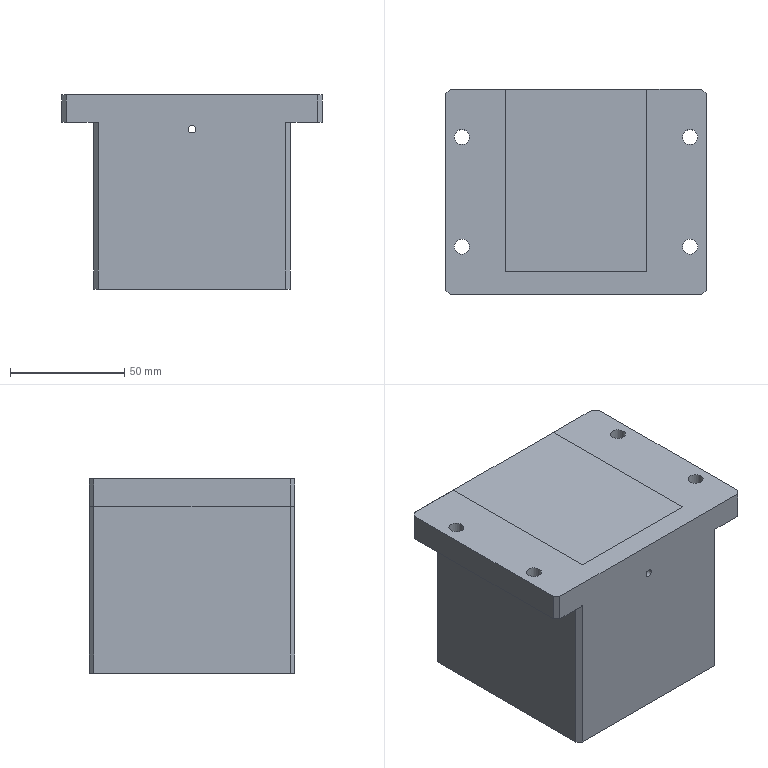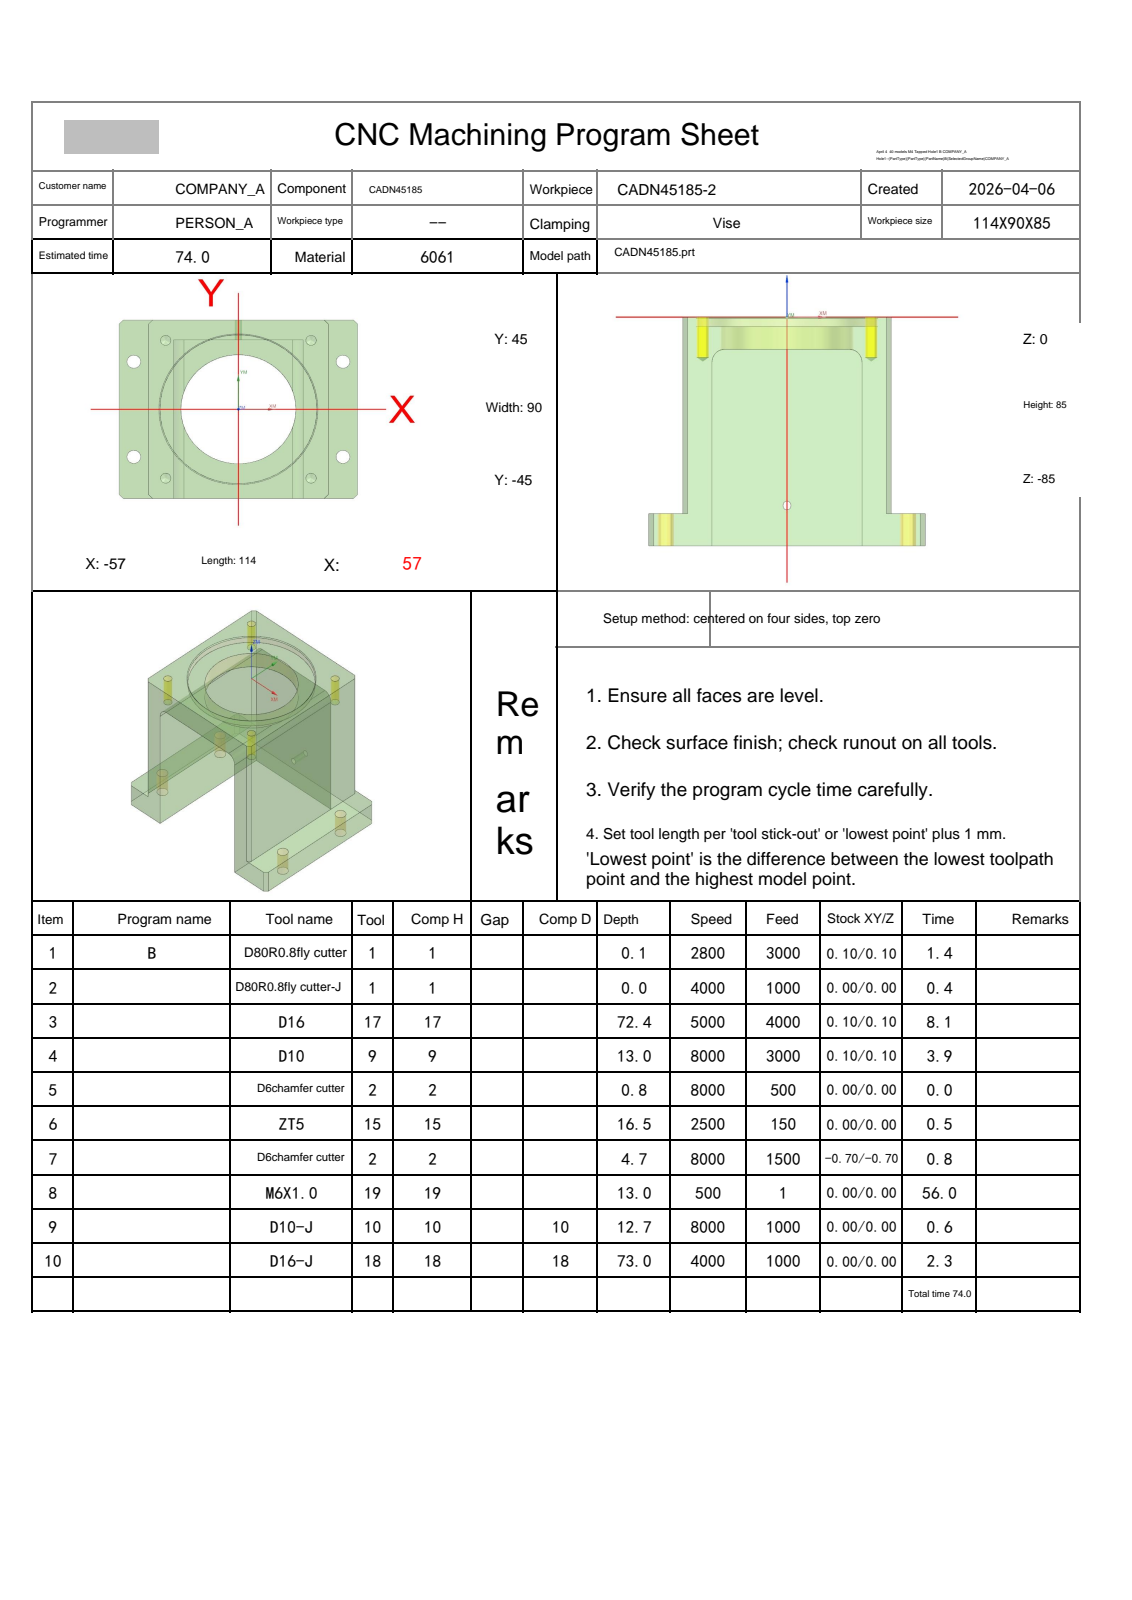NC program | NX | posted by the shop | part box 114 x 90 x 85 mm
Lines 2097 to 3620 of 3620:
N4 T09 M06
(D10  D=10. R=0. H=09 ce=0.10 di=0.10)
G00 G90 G54 X30.162 Y3.101 M03 S8000
G43 H09 Z14.5
M08
Z1.5
G02 X30.162 Y3.101 Z1.006 I-3.261 J-3.101 F3000.
X30.162 Y3.101 Z.513 I-3.261 J-3.101
X30.162 Y3.101 Z.019 I-3.261 J-3.101
X30.162 Y3.101 Z-.474 I-3.261 J-3.101
X30.583 Y2.587 Z-.486 I-3.261 J-3.101
G01 X32.401 Y0.0
G02 X0.0 Y-32.401 I-32.401 J0.0
X-32.401 Y0.0 I0.0 J32.401
X0.0 Y32.401 I32.401 J0.0
X32.401 Y0.0 I0.0 J-32.401
X32.12 Y-4.259 I-32.401 J0.0
X31.311 Y-5.111 I-.991 J.132
G01 X25.212 Y-6.237
G03 X24.433 Y-6.947 I.182 J-.983
G02 X0.0 Y-25.401 I-24.433 J6.947
X-25.401 Y0.0 I0.0 J25.401
X0.0 Y25.401 I25.401 J0.0
X25.401 Y0.0 I0.0 J-25.401
X25.388 Y-.819 I-25.401 J0.0
X24.834 Y-1.681 I-.999 J.033
G01 X18.014 Y-5.075
G03 X17.508 Y-5.662 I.446 J-.895
G02 X0.0 Y-18.401 I-17.508 J5.662
X-18.401 Y0.0 I0.0 J18.401
X0.0 Y18.401 I18.401 J0.0
X18.399 Y.3 I0.0 J-18.401
G01 Y.284
G02 X17.84 Y-.614 I-1. J0.0
G01 X10.955 Y-3.994
G03 X10.477 Y-4.497 I.441 J-.898
G02 X0.0 Y-11.401 I-10.477 J4.497
X-11.401 Y0.0 I0.0 J11.401
X0.0 Y11.401 I11.401 J0.0
X11.304 Y1.486 I0.0 J-11.401
G01 X11.312 Y1.356
G02 X10.724 Y.445 I-1. J0.0
G01 X3.487 Y-2.826
G03 X3.178 Y-3.045 I.412 J-.911
G02 X0.0 Y-4.401 I-3.178 J3.045
X-4.401 Y0.0 I0.0 J4.401
X0.0 Y4.401 I4.401 J0.0
X4.401 Y0.0 I0.0 J-4.401
X4.349 Y-.676 I-4.401 J0.0
X4.244 Y-1.165 I-4.349 J.676
G03 X3.994 Y-3.018 I6.75 J-1.853
X9.141 Y-9.768 I7. J0.0
G01 Z.714
G00 Z3.
G01 X30.161 Y3.101 F6000.
G00 Z1.014
G02 X30.161 Y3.101 Z.521 I-3.261 J-3.101 F3000.
X30.161 Y3.101 Z.027 I-3.261 J-3.101
X30.161 Y3.101 Z-.466 I-3.261 J-3.101
X30.161 Y3.101 Z-.96 I-3.261 J-3.101
X30.582 Y2.587 Z-.971 I-3.261 J-3.101
G01 X32.4 Y0.0
G02 X0.0 Y-32.4 I-32.4 J0.0
X-32.4 Y0.0 I0.0 J32.4
X0.0 Y32.4 I32.4 J0.0
X32.4 Y0.0 I0.0 J-32.4
X32.015 Y-4.98 I-32.4 J0.0
X31.108 Y-5.823 I-.988 J.154
G01 X25.292 Y-6.295
G03 X24.412 Y-7.015 I.081 J-.997
G02 X0.0 Y-25.4 I-24.412 J7.015
X-25.4 Y0.0 I0.0 J25.4
X0.0 Y25.4 I25.4 J0.0
X25.4 Y0.0 I0.0 J-25.4
X25.387 Y-.819 I-25.4 J0.0
X24.833 Y-1.681 I-.999 J.033
G01 X18.013 Y-5.075
G03 X17.507 Y-5.662 I.446 J-.895
G02 X0.0 Y-18.4 I-17.507 J5.662
X-18.4 Y0.0 I0.0 J18.4
X0.0 Y18.4 I18.4 J0.0
X18.398 Y.3 I0.0 J-18.4
G01 Y.284
G02 X17.839 Y-.614 I-1. J0.0
G01 X10.953 Y-3.994
G03 X10.476 Y-4.497 I.441 J-.897
G02 X0.0 Y-11.4 I-10.476 J4.497
X-11.4 Y0.0 I0.0 J11.4
X0.0 Y11.4 I11.4 J0.0
X11.303 Y1.486 I0.0 J-11.4
G01 X11.311 Y1.356
G02 X10.723 Y.445 I-1. J0.0
G01 X3.486 Y-2.826
G03 X3.176 Y-3.045 I.412 J-.911
G02 X0.0 Y-4.4 I-3.176 J3.045
X-4.4 Y0.0 I0.0 J4.4
X0.0 Y4.4 I4.4 J0.0
X4.4 Y0.0 I0.0 J-4.4
X4.348 Y-.676 I-4.4 J0.0
X4.243 Y-1.165 I-4.348 J.676
G03 X3.993 Y-3.018 I6.75 J-1.853
X9.14 Y-9.768 I7. J0.0
G01 Z.229
G00 Z2.514
G01 X30.161 Y3.101 F6000.
G00 Z.529
G02 X30.161 Y3.101 Z.035 I-3.261 J-3.101 F3000.
X30.161 Y3.101 Z-.458 I-3.261 J-3.101
X30.161 Y3.101 Z-.952 I-3.261 J-3.101
X30.161 Y3.101 Z-1.446 I-3.261 J-3.101
X30.582 Y2.587 Z-1.457 I-3.261 J-3.101
G01 X32.4 Y0.0
G02 X0.0 Y-32.4 I-32.4 J0.0
X-32.4 Y0.0 I0.0 J32.4
X0.0 Y32.4 I32.4 J0.0
X32.4 Y0.0 I0.0 J-32.4
X32.015 Y-4.98 I-32.4 J0.0
X31.108 Y-5.823 I-.988 J.154
G01 X25.292 Y-6.295
G03 X24.412 Y-7.015 I.081 J-.997
G02 X0.0 Y-25.4 I-24.412 J7.015
X-25.4 Y0.0 I0.0 J25.4
X0.0 Y25.4 I25.4 J0.0
X25.4 Y0.0 I0.0 J-25.4
X25.387 Y-.819 I-25.4 J0.0
X24.833 Y-1.681 I-.999 J.033
G01 X18.013 Y-5.075
G03 X17.507 Y-5.662 I.446 J-.895
G02 X0.0 Y-18.4 I-17.507 J5.662
X-18.4 Y0.0 I0.0 J18.4
X0.0 Y18.4 I18.4 J0.0
X18.398 Y.3 I0.0 J-18.4
G01 Y.284
G02 X17.839 Y-.614 I-1. J0.0
G01 X10.953 Y-3.994
G03 X10.476 Y-4.497 I.441 J-.897
G02 X0.0 Y-11.4 I-10.476 J4.497
X-11.4 Y0.0 I0.0 J11.4
X0.0 Y11.4 I11.4 J0.0
X11.303 Y1.486 I0.0 J-11.4
G01 X11.311 Y1.356
G02 X10.723 Y.445 I-1. J0.0
G01 X3.486 Y-2.826
G03 X3.176 Y-3.045 I.412 J-.911
G02 X0.0 Y-4.4 I-3.176 J3.045
X-4.4 Y0.0 I0.0 J4.4
X0.0 Y4.4 I4.4 J0.0
X4.4 Y0.0 I0.0 J-4.4
X4.348 Y-.676 I-4.4 J0.0
X4.243 Y-1.165 I-4.348 J.676
G03 X3.993 Y-3.018 I6.75 J-1.853
X9.14 Y-9.768 I7. J0.0
G01 Z-.257
G00 Z2.029
G01 X30.161 Y3.101 F6000.
G00 Z.043
G02 X30.161 Y3.101 Z-.451 I-3.261 J-3.101 F3000.
X30.161 Y3.101 Z-.944 I-3.261 J-3.101
X30.161 Y3.101 Z-1.438 I-3.261 J-3.101
X30.161 Y3.101 Z-1.931 I-3.261 J-3.101
X30.582 Y2.587 Z-1.943 I-3.261 J-3.101
G01 X32.4 Y0.0
G02 X0.0 Y-32.4 I-32.4 J0.0
X-32.4 Y0.0 I0.0 J32.4
X0.0 Y32.4 I32.4 J0.0
X32.4 Y0.0 I0.0 J-32.4
X32.015 Y-4.98 I-32.4 J0.0
X31.108 Y-5.823 I-.988 J.154
G01 X25.292 Y-6.295
G03 X24.412 Y-7.015 I.081 J-.997
G02 X0.0 Y-25.4 I-24.412 J7.015
X-25.4 Y0.0 I0.0 J25.4
X0.0 Y25.4 I25.4 J0.0
X25.4 Y0.0 I0.0 J-25.4
X25.387 Y-.819 I-25.4 J0.0
X24.833 Y-1.681 I-.999 J.033
G01 X18.013 Y-5.075
G03 X17.507 Y-5.662 I.446 J-.895
G02 X0.0 Y-18.4 I-17.507 J5.662
X-18.4 Y0.0 I0.0 J18.4
X0.0 Y18.4 I18.4 J0.0
X18.398 Y.3 I0.0 J-18.4
G01 Y.284
G02 X17.839 Y-.614 I-1. J0.0
G01 X10.953 Y-3.994
G03 X10.476 Y-4.497 I.441 J-.897
G02 X0.0 Y-11.4 I-10.476 J4.497
X-11.4 Y0.0 I0.0 J11.4
X0.0 Y11.4 I11.4 J0.0
X11.303 Y1.486 I0.0 J-11.4
G01 X11.311 Y1.356
G02 X10.723 Y.445 I-1. J0.0
G01 X3.486 Y-2.826
G03 X3.176 Y-3.045 I.412 J-.911
G02 X0.0 Y-4.4 I-3.176 J3.045
X-4.4 Y0.0 I0.0 J4.4
X0.0 Y4.4 I4.4 J0.0
X4.4 Y0.0 I0.0 J-4.4
X4.348 Y-.676 I-4.4 J0.0
X4.243 Y-1.165 I-4.348 J.676
G03 X3.993 Y-3.018 I6.75 J-1.853
X9.14 Y-9.768 I7. J0.0
G01 Z-.743
G00 Z1.543
G01 X30.161 Y3.101 F6000.
G00 Z-.443
G02 X30.161 Y3.101 Z-.936 I-3.261 J-3.101 F3000.
X30.161 Y3.101 Z-1.43 I-3.261 J-3.101
X30.161 Y3.101 Z-1.923 I-3.261 J-3.101
X30.161 Y3.101 Z-2.417 I-3.261 J-3.101
X30.582 Y2.587 Z-2.429 I-3.261 J-3.101
G01 X32.4 Y0.0
G02 X0.0 Y-32.4 I-32.4 J0.0
X-32.4 Y0.0 I0.0 J32.4
X0.0 Y32.4 I32.4 J0.0
X32.4 Y0.0 I0.0 J-32.4
X32.015 Y-4.98 I-32.4 J0.0
X31.108 Y-5.823 I-.988 J.154
G01 X25.292 Y-6.295
G03 X24.412 Y-7.015 I.081 J-.997
G02 X0.0 Y-25.4 I-24.412 J7.015
X-25.4 Y0.0 I0.0 J25.4
X0.0 Y25.4 I25.4 J0.0
X25.4 Y0.0 I0.0 J-25.4
X25.387 Y-.819 I-25.4 J0.0
X24.833 Y-1.681 I-.999 J.033
G01 X18.013 Y-5.075
G03 X17.507 Y-5.662 I.446 J-.895
G02 X0.0 Y-18.4 I-17.507 J5.662
X-18.4 Y0.0 I0.0 J18.4
X0.0 Y18.4 I18.4 J0.0
X18.398 Y.3 I0.0 J-18.4
G01 Y.284
G02 X17.839 Y-.614 I-1. J0.0
G01 X10.953 Y-3.994
G03 X10.476 Y-4.497 I.441 J-.897
G02 X0.0 Y-11.4 I-10.476 J4.497
X-11.4 Y0.0 I0.0 J11.4
X0.0 Y11.4 I11.4 J0.0
X11.303 Y1.486 I0.0 J-11.4
G01 X11.311 Y1.356
G02 X10.723 Y.445 I-1. J0.0
G01 X3.486 Y-2.826
G03 X3.176 Y-3.045 I.412 J-.911
G02 X0.0 Y-4.4 I-3.176 J3.045
X-4.4 Y0.0 I0.0 J4.4
X0.0 Y4.4 I4.4 J0.0
X4.4 Y0.0 I0.0 J-4.4
X4.348 Y-.676 I-4.4 J0.0
X4.243 Y-1.165 I-4.348 J.676
G03 X3.993 Y-3.018 I6.75 J-1.853
X9.14 Y-9.768 I7. J0.0
G01 Z-1.229
G00 Z1.057
G01 X30.161 Y3.101 F6000.
G00 Z-.929
G02 X30.161 Y3.101 Z-1.422 I-3.261 J-3.101 F3000.
X30.161 Y3.101 Z-1.916 I-3.261 J-3.101
X30.161 Y3.101 Z-2.409 I-3.261 J-3.101
X30.161 Y3.101 Z-2.903 I-3.261 J-3.101
X30.582 Y2.587 Z-2.914 I-3.261 J-3.101
G01 X32.4 Y0.0
G02 X0.0 Y-32.4 I-32.4 J0.0
X-32.4 Y0.0 I0.0 J32.4
X0.0 Y32.4 I32.4 J0.0
X32.4 Y0.0 I0.0 J-32.4
X32.015 Y-4.98 I-32.4 J0.0
X31.108 Y-5.823 I-.988 J.154
G01 X25.292 Y-6.295
G03 X24.412 Y-7.015 I.081 J-.997
G02 X0.0 Y-25.4 I-24.412 J7.015
X-25.4 Y0.0 I0.0 J25.4
X0.0 Y25.4 I25.4 J0.0
X25.4 Y0.0 I0.0 J-25.4
X25.387 Y-.819 I-25.4 J0.0
X24.833 Y-1.681 I-.999 J.033
G01 X18.013 Y-5.075
G03 X17.507 Y-5.662 I.446 J-.895
G02 X0.0 Y-18.4 I-17.507 J5.662
X-18.4 Y0.0 I0.0 J18.4
X0.0 Y18.4 I18.4 J0.0
X18.398 Y.3 I0.0 J-18.4
G01 Y.284
G02 X17.839 Y-.614 I-1. J0.0
G01 X10.953 Y-3.994
G03 X10.476 Y-4.497 I.441 J-.897
G02 X0.0 Y-11.4 I-10.476 J4.497
X-11.4 Y0.0 I0.0 J11.4
X0.0 Y11.4 I11.4 J0.0
X11.303 Y1.486 I0.0 J-11.4
G01 X11.311 Y1.356
G02 X10.723 Y.445 I-1. J0.0
G01 X3.486 Y-2.826
G03 X3.176 Y-3.045 I.412 J-.911
G02 X0.0 Y-4.4 I-3.176 J3.045
X-4.4 Y0.0 I0.0 J4.4
X0.0 Y4.4 I4.4 J0.0
X4.4 Y0.0 I0.0 J-4.4
X4.348 Y-.676 I-4.4 J0.0
X4.243 Y-1.165 I-4.348 J.676
G03 X3.993 Y-3.018 I6.75 J-1.853
X9.14 Y-9.768 I7. J0.0
G01 Z-1.714
G00 Z.571
G01 X30.161 Y3.101 F6000.
G00 Z-1.414
G02 X30.161 Y3.101 Z-1.908 I-3.261 J-3.101 F3000.
X30.161 Y3.101 Z-2.401 I-3.261 J-3.101
X30.161 Y3.101 Z-2.895 I-3.261 J-3.101
X30.161 Y3.101 Z-3.388 I-3.261 J-3.101
X30.582 Y2.587 Z-3.4 I-3.261 J-3.101
G01 X32.4 Y0.0
G02 X0.0 Y-32.4 I-32.4 J0.0
X-32.4 Y0.0 I0.0 J32.4
X0.0 Y32.4 I32.4 J0.0
X32.4 Y0.0 I0.0 J-32.4
X32.015 Y-4.98 I-32.4 J0.0
X31.108 Y-5.823 I-.988 J.154
G01 X25.292 Y-6.295
G03 X24.412 Y-7.015 I.081 J-.997
G02 X0.0 Y-25.4 I-24.412 J7.015
X-25.4 Y0.0 I0.0 J25.4
X0.0 Y25.4 I25.4 J0.0
X25.4 Y0.0 I0.0 J-25.4
X25.387 Y-.819 I-25.4 J0.0
X24.833 Y-1.681 I-.999 J.033
G01 X18.013 Y-5.075
G03 X17.507 Y-5.662 I.446 J-.895
G02 X0.0 Y-18.4 I-17.507 J5.662
X-18.4 Y0.0 I0.0 J18.4
X0.0 Y18.4 I18.4 J0.0
X18.398 Y.3 I0.0 J-18.4
G01 Y.284
G02 X17.839 Y-.614 I-1. J0.0
G01 X10.953 Y-3.994
G03 X10.476 Y-4.497 I.441 J-.897
G02 X0.0 Y-11.4 I-10.476 J4.497
X-11.4 Y0.0 I0.0 J11.4
X0.0 Y11.4 I11.4 J0.0
X11.303 Y1.486 I0.0 J-11.4
G01 X11.311 Y1.356
G02 X10.723 Y.445 I-1. J0.0
G01 X3.486 Y-2.826
G03 X3.176 Y-3.045 I.412 J-.911
G02 X0.0 Y-4.4 I-3.176 J3.045
X-4.4 Y0.0 I0.0 J4.4
X0.0 Y4.4 I4.4 J0.0
X4.4 Y0.0 I0.0 J-4.4
X4.348 Y-.676 I-4.4 J0.0
X4.243 Y-1.165 I-4.348 J.676
G03 X3.993 Y-3.018 I6.75 J-1.853
X9.14 Y-9.768 I7. J0.0
G01 Z-2.2
G00 Z.086
G01 X-.738 Y-12.461 F6000.
G00 Z-1.9
G02 X-.738 Y-12.461 Z-2.394 I.738 J-4.439 F3000.
X-.738 Y-12.461 Z-2.887 I.738 J-4.439
X-.738 Y-12.461 Z-3.381 I.738 J-4.439
X-.738 Y-12.461 Z-3.874 I.738 J-4.439
X2.587 Y-20.582 Z-4.086 I.738 J-4.439
G01 X0.0 Y-22.4
G02 X-22.4 Y0.0 I0.0 J22.4
X0.0 Y22.4 I22.4 J0.0
X22.4 Y0.0 I0.0 J-22.4
X0.0 Y-22.4 I-22.4 J0.0
X-4.959 Y-21.844 I0.0 J22.4
X-5.737 Y-20.877 I.221 J.975
G01 X-5.786 Y-14.922
G03 X-6.372 Y-14.02 I-1. J-.009
G02 X-15.4 Y0.0 I6.372 J14.02
X0.0 Y15.4 I15.4 J0.0
X15.4 Y0.0 I0.0 J-15.4
X0.0 Y-15.4 I-15.4 J0.0
X-.268 Y-15.398 I0.0 J15.4
X-1.178 Y-14.77 I.018 J1.
G01 X-4.055 Y-7.598
G03 X-4.452 Y-7.123 I-.928 J-.373
G02 X-8.4 Y0.0 I4.452 J7.123
X0.0 Y8.4 I8.4 J0.0
X8.4 Y0.0 I0.0 J-8.4
X1.562 Y-8.254 I-8.4 J0.0
G01 X1.395 Y-8.269
G02 X.503 Y-7.492 I0.0 J.9
G01 X-.264 Y-1.91
G03 X-.731 Y-1.194 I-.991 J-.136
G02 X-1.4 Y0.0 I.731 J1.194
X0.0 Y1.4 I1.4 J0.0
X1.4 Y0.0 I0.0 J-1.4
X0.0 Y-1.4 I-1.4 J0.0
X-.31 Y-1.365 I0.0 J1.4
G01 X-.339 Y-1.358
G02 X-.768 Y-1.171 I.339 J1.358
G03 X-4.606 Y-.025 I-3.838 J-5.854
X-10.46 Y-3.186 I0.0 J-7.
G01 Z-2.886
G00 Z-.4
G01 X-.738 Y-12.461 F6000.
G00 Z-2.586
G02 X-.738 Y-12.461 Z-3.079 I.738 J-4.439 F3000.
X-.738 Y-12.461 Z-3.573 I.738 J-4.439
X-.738 Y-12.461 Z-4.066 I.738 J-4.439
X-.738 Y-12.461 Z-4.56 I.738 J-4.439
X2.587 Y-20.582 Z-4.771 I.738 J-4.439
G01 X0.0 Y-22.4
G02 X-22.4 Y0.0 I0.0 J22.4
X0.0 Y22.4 I22.4 J0.0
X22.4 Y0.0 I0.0 J-22.4
X0.0 Y-22.4 I-22.4 J0.0
X-4.959 Y-21.844 I0.0 J22.4
X-5.737 Y-20.877 I.221 J.975
G01 X-5.786 Y-14.922
G03 X-6.372 Y-14.02 I-1. J-.009
G02 X-15.4 Y0.0 I6.372 J14.02
X0.0 Y15.4 I15.4 J0.0
X15.4 Y0.0 I0.0 J-15.4
X0.0 Y-15.4 I-15.4 J0.0
X-.268 Y-15.398 I0.0 J15.4
X-1.178 Y-14.77 I.018 J1.
G01 X-4.055 Y-7.598
G03 X-4.452 Y-7.123 I-.928 J-.373
G02 X-8.4 Y0.0 I4.452 J7.123
X0.0 Y8.4 I8.4 J0.0
X8.4 Y0.0 I0.0 J-8.4
X1.562 Y-8.254 I-8.4 J0.0
G01 X1.395 Y-8.269
G02 X.503 Y-7.492 I0.0 J.9
G01 X-.264 Y-1.91
G03 X-.731 Y-1.194 I-.991 J-.136
G02 X-1.4 Y0.0 I.731 J1.194
X0.0 Y1.4 I1.4 J0.0
X1.4 Y0.0 I0.0 J-1.4
X0.0 Y-1.4 I-1.4 J0.0
X-.31 Y-1.365 I0.0 J1.4
G01 X-.339 Y-1.358
G02 X-.768 Y-1.171 I.339 J1.358
G03 X-4.606 Y-.025 I-3.838 J-5.854
X-10.46 Y-3.186 I0.0 J-7.
G01 Z-3.571
G00 Z-1.086
G01 X-.738 Y-12.461 F6000.
G00 Z-3.271
G02 X-.738 Y-12.461 Z-3.765 I.738 J-4.439 F3000.
X-.738 Y-12.461 Z-4.258 I.738 J-4.439
X-.738 Y-12.461 Z-4.752 I.738 J-4.439
X-.738 Y-12.461 Z-5.246 I.738 J-4.439
X2.587 Y-20.582 Z-5.457 I.738 J-4.439
G01 X0.0 Y-22.4
G02 X-22.4 Y0.0 I0.0 J22.4
X0.0 Y22.4 I22.4 J0.0
X22.4 Y0.0 I0.0 J-22.4
X0.0 Y-22.4 I-22.4 J0.0
X-4.959 Y-21.844 I0.0 J22.4
X-5.737 Y-20.877 I.221 J.975
G01 X-5.786 Y-14.922
G03 X-6.372 Y-14.02 I-1. J-.009
G02 X-15.4 Y0.0 I6.372 J14.02
X0.0 Y15.4 I15.4 J0.0
X15.4 Y0.0 I0.0 J-15.4
X0.0 Y-15.4 I-15.4 J0.0
X-.268 Y-15.398 I0.0 J15.4
X-1.178 Y-14.77 I.018 J1.
G01 X-4.055 Y-7.598
G03 X-4.452 Y-7.123 I-.928 J-.373
G02 X-8.4 Y0.0 I4.452 J7.123
X0.0 Y8.4 I8.4 J0.0
X8.4 Y0.0 I0.0 J-8.4
X1.562 Y-8.254 I-8.4 J0.0
G01 X1.395 Y-8.269
G02 X.503 Y-7.492 I0.0 J.9
G01 X-.264 Y-1.91
G03 X-.731 Y-1.194 I-.991 J-.136
G02 X-1.4 Y0.0 I.731 J1.194
X0.0 Y1.4 I1.4 J0.0
X1.4 Y0.0 I0.0 J-1.4
X0.0 Y-1.4 I-1.4 J0.0
X-.31 Y-1.365 I0.0 J1.4
G01 X-.339 Y-1.358
G02 X-.768 Y-1.171 I.339 J1.358
G03 X-4.606 Y-.025 I-3.838 J-5.854
X-10.46 Y-3.186 I0.0 J-7.
G01 Z-4.257
G00 Z-1.771
G01 X-.738 Y-12.461 F6000.
G00 Z-3.957
G02 X-.738 Y-12.461 Z-4.451 I.738 J-4.439 F3000.
X-.738 Y-12.461 Z-4.944 I.738 J-4.439
X-.738 Y-12.461 Z-5.438 I.738 J-4.439
X-.738 Y-12.461 Z-5.931 I.738 J-4.439
X2.587 Y-20.582 Z-6.143 I.738 J-4.439
G01 X0.0 Y-22.4
G02 X-22.4 Y0.0 I0.0 J22.4
X0.0 Y22.4 I22.4 J0.0
X22.4 Y0.0 I0.0 J-22.4
X0.0 Y-22.4 I-22.4 J0.0
X-4.959 Y-21.844 I0.0 J22.4
X-5.737 Y-20.877 I.221 J.975
G01 X-5.786 Y-14.922
G03 X-6.372 Y-14.02 I-1. J-.009
G02 X-15.4 Y0.0 I6.372 J14.02
X0.0 Y15.4 I15.4 J0.0
X15.4 Y0.0 I0.0 J-15.4
X0.0 Y-15.4 I-15.4 J0.0
X-.268 Y-15.398 I0.0 J15.4
X-1.178 Y-14.77 I.018 J1.
G01 X-4.055 Y-7.598
G03 X-4.452 Y-7.123 I-.928 J-.373
G02 X-8.4 Y0.0 I4.452 J7.123
X0.0 Y8.4 I8.4 J0.0
X8.4 Y0.0 I0.0 J-8.4
X1.562 Y-8.254 I-8.4 J0.0
G01 X1.395 Y-8.269
G02 X.503 Y-7.492 I0.0 J.9
G01 X-.264 Y-1.91
G03 X-.731 Y-1.194 I-.991 J-.136
G02 X-1.4 Y0.0 I.731 J1.194
X0.0 Y1.4 I1.4 J0.0
X1.4 Y0.0 I0.0 J-1.4
X0.0 Y-1.4 I-1.4 J0.0
X-.31 Y-1.365 I0.0 J1.4
G01 X-.339 Y-1.358
G02 X-.768 Y-1.171 I.339 J1.358
G03 X-4.606 Y-.025 I-3.838 J-5.854
X-10.46 Y-3.186 I0.0 J-7.
G01 Z-4.943
G00 Z-2.457
G01 X-.738 Y-12.461 F6000.
G00 Z-4.643
G02 X-.738 Y-12.461 Z-5.136 I.738 J-4.439 F3000.
X-.738 Y-12.461 Z-5.63 I.738 J-4.439
X-.738 Y-12.461 Z-6.123 I.738 J-4.439
X-.738 Y-12.461 Z-6.617 I.738 J-4.439
X2.587 Y-20.582 Z-6.829 I.738 J-4.439
G01 X0.0 Y-22.4
G02 X-22.4 Y0.0 I0.0 J22.4
X0.0 Y22.4 I22.4 J0.0
X22.4 Y0.0 I0.0 J-22.4
X0.0 Y-22.4 I-22.4 J0.0
X-4.959 Y-21.844 I0.0 J22.4
X-5.737 Y-20.877 I.221 J.975
G01 X-5.786 Y-14.922
G03 X-6.372 Y-14.02 I-1. J-.009
G02 X-15.4 Y0.0 I6.372 J14.02
X0.0 Y15.4 I15.4 J0.0
X15.4 Y0.0 I0.0 J-15.4
X0.0 Y-15.4 I-15.4 J0.0
X-.268 Y-15.398 I0.0 J15.4
X-1.178 Y-14.77 I.018 J1.
G01 X-4.055 Y-7.598
G03 X-4.452 Y-7.123 I-.928 J-.373
G02 X-8.4 Y0.0 I4.452 J7.123
X0.0 Y8.4 I8.4 J0.0
X8.4 Y0.0 I0.0 J-8.4
X1.562 Y-8.254 I-8.4 J0.0
G01 X1.395 Y-8.269
G02 X.503 Y-7.492 I0.0 J.9
G01 X-.264 Y-1.91
G03 X-.731 Y-1.194 I-.991 J-.136
G02 X-1.4 Y0.0 I.731 J1.194
X0.0 Y1.4 I1.4 J0.0
X1.4 Y0.0 I0.0 J-1.4
X0.0 Y-1.4 I-1.4 J0.0
X-.31 Y-1.365 I0.0 J1.4
G01 X-.339 Y-1.358
G02 X-.768 Y-1.171 I.339 J1.358
G03 X-4.606 Y-.025 I-3.838 J-5.854
X-10.46 Y-3.186 I0.0 J-7.
G01 Z-5.629
G00 Z-3.143
G01 X-.738 Y-12.461 F6000.
G00 Z-5.329
G02 X-.738 Y-12.461 Z-5.822 I.738 J-4.439 F3000.
X-.738 Y-12.461 Z-6.316 I.738 J-4.439
X-.738 Y-12.461 Z-6.809 I.738 J-4.439
X-.738 Y-12.461 Z-7.303 I.738 J-4.439
X2.587 Y-20.582 Z-7.514 I.738 J-4.439
G01 X0.0 Y-22.4
G02 X-22.4 Y0.0 I0.0 J22.4
X0.0 Y22.4 I22.4 J0.0
X22.4 Y0.0 I0.0 J-22.4
X0.0 Y-22.4 I-22.4 J0.0
X-4.959 Y-21.844 I0.0 J22.4
X-5.737 Y-20.877 I.221 J.975
G01 X-5.786 Y-14.922
G03 X-6.372 Y-14.02 I-1. J-.009
G02 X-15.4 Y0.0 I6.372 J14.02
X0.0 Y15.4 I15.4 J0.0
X15.4 Y0.0 I0.0 J-15.4
X0.0 Y-15.4 I-15.4 J0.0
X-.268 Y-15.398 I0.0 J15.4
X-1.178 Y-14.77 I.018 J1.
G01 X-4.055 Y-7.598
G03 X-4.452 Y-7.123 I-.928 J-.373
G02 X-8.4 Y0.0 I4.452 J7.123
X0.0 Y8.4 I8.4 J0.0
X8.4 Y0.0 I0.0 J-8.4
X1.562 Y-8.254 I-8.4 J0.0
G01 X1.395 Y-8.269
G02 X.503 Y-7.492 I0.0 J.9
G01 X-.264 Y-1.91
G03 X-.731 Y-1.194 I-.991 J-.136
G02 X-1.4 Y0.0 I.731 J1.194
X0.0 Y1.4 I1.4 J0.0
X1.4 Y0.0 I0.0 J-1.4
X0.0 Y-1.4 I-1.4 J0.0
X-.31 Y-1.365 I0.0 J1.4
G01 X-.339 Y-1.358
G02 X-.768 Y-1.171 I.339 J1.358
G03 X-4.606 Y-.025 I-3.838 J-5.854
X-10.46 Y-3.186 I0.0 J-7.
G01 Z-6.314
G00 Z-3.829
G01 X-.738 Y-12.461 F6000.
G00 Z-6.014
G02 X-.738 Y-12.461 Z-6.508 I.738 J-4.439 F3000.
X-.738 Y-12.461 Z-7.001 I.738 J-4.439
X-.738 Y-12.461 Z-7.495 I.738 J-4.439
X-.738 Y-12.461 Z-7.988 I.738 J-4.439
X2.587 Y-20.582 Z-8.2 I.738 J-4.439
G01 X0.0 Y-22.4
G02 X-22.4 Y0.0 I0.0 J22.4
X0.0 Y22.4 I22.4 J0.0
X22.4 Y0.0 I0.0 J-22.4
X0.0 Y-22.4 I-22.4 J0.0
X-4.959 Y-21.844 I0.0 J22.4
X-5.737 Y-20.877 I.221 J.975
G01 X-5.786 Y-14.922
G03 X-6.372 Y-14.02 I-1. J-.009
G02 X-15.4 Y0.0 I6.372 J14.02
X0.0 Y15.4 I15.4 J0.0
X15.4 Y0.0 I0.0 J-15.4
X0.0 Y-15.4 I-15.4 J0.0
X-.268 Y-15.398 I0.0 J15.4
X-1.178 Y-14.77 I.018 J1.
G01 X-4.055 Y-7.598
G03 X-4.452 Y-7.123 I-.928 J-.373
G02 X-8.4 Y0.0 I4.452 J7.123
X0.0 Y8.4 I8.4 J0.0
X8.4 Y0.0 I0.0 J-8.4
X1.562 Y-8.254 I-8.4 J0.0
G01 X1.395 Y-8.269
G02 X.503 Y-7.492 I0.0 J.9
G01 X-.264 Y-1.91
G03 X-.731 Y-1.194 I-.991 J-.136
G02 X-1.4 Y0.0 I.731 J1.194
X0.0 Y1.4 I1.4 J0.0
X1.4 Y0.0 I0.0 J-1.4
X0.0 Y-1.4 I-1.4 J0.0
X-.31 Y-1.365 I0.0 J1.4
G01 X-.339 Y-1.358
G02 X-.768 Y-1.171 I.339 J1.358
G03 X-4.606 Y-.025 I-3.838 J-5.854
X-10.46 Y-3.186 I0.0 J-7.
G01 Z-7.
G00 Z-4.514
G01 X-.738 Y-12.461 F6000.
G00 Z-6.7
G02 X-.738 Y-12.461 Z-7.194 I.738 J-4.439 F3000.
X-.738 Y-12.461 Z-7.687 I.738 J-4.439
X-.738 Y-12.461 Z-8.181 I.738 J-4.439
X-.738 Y-12.461 Z-8.674 I.738 J-4.439
X2.587 Y-20.582 Z-8.886 I.738 J-4.439
G01 X0.0 Y-22.4
G02 X-22.4 Y0.0 I0.0 J22.4
X0.0 Y22.4 I22.4 J0.0
X22.4 Y0.0 I0.0 J-22.4
X0.0 Y-22.4 I-22.4 J0.0
X-4.959 Y-21.844 I0.0 J22.4
X-5.737 Y-20.877 I.221 J.975
G01 X-5.786 Y-14.922
G03 X-6.372 Y-14.02 I-1. J-.009
G02 X-15.4 Y0.0 I6.372 J14.02
X0.0 Y15.4 I15.4 J0.0
X15.4 Y0.0 I0.0 J-15.4
X0.0 Y-15.4 I-15.4 J0.0
X-.268 Y-15.398 I0.0 J15.4
X-1.178 Y-14.77 I.018 J1.
G01 X-4.055 Y-7.598
G03 X-4.452 Y-7.123 I-.928 J-.373
G02 X-8.4 Y0.0 I4.452 J7.123
X0.0 Y8.4 I8.4 J0.0
X8.4 Y0.0 I0.0 J-8.4
X1.562 Y-8.254 I-8.4 J0.0
G01 X1.395 Y-8.269
G02 X.503 Y-7.492 I0.0 J.9
G01 X-.264 Y-1.91
G03 X-.731 Y-1.194 I-.991 J-.136
G02 X-1.4 Y0.0 I.731 J1.194
X0.0 Y1.4 I1.4 J0.0
X1.4 Y0.0 I0.0 J-1.4
X0.0 Y-1.4 I-1.4 J0.0
X-.31 Y-1.365 I0.0 J1.4
G01 X-.339 Y-1.358
G02 X-.768 Y-1.171 I.339 J1.358
G03 X-4.606 Y-.025 I-3.838 J-5.854
X-10.46 Y-3.186 I0.0 J-7.
G01 Z-7.686
G00 Z-5.2
G01 X-.738 Y-12.461 F6000.
G00 Z-7.386
G02 X-.738 Y-12.461 Z-7.879 I.738 J-4.439 F3000.
X-.738 Y-12.461 Z-8.373 I.738 J-4.439
X-.738 Y-12.461 Z-8.866 I.738 J-4.439
X-.738 Y-12.461 Z-9.36 I.738 J-4.439
X2.587 Y-20.582 Z-9.571 I.738 J-4.439
G01 X0.0 Y-22.4
G02 X-22.4 Y0.0 I0.0 J22.4
X0.0 Y22.4 I22.4 J0.0
X22.4 Y0.0 I0.0 J-22.4
X0.0 Y-22.4 I-22.4 J0.0
X-4.959 Y-21.844 I0.0 J22.4
X-5.737 Y-20.877 I.221 J.975
G01 X-5.786 Y-14.922
G03 X-6.372 Y-14.02 I-1. J-.009
G02 X-15.4 Y0.0 I6.372 J14.02
X0.0 Y15.4 I15.4 J0.0
X15.4 Y0.0 I0.0 J-15.4
X0.0 Y-15.4 I-15.4 J0.0
X-.268 Y-15.398 I0.0 J15.4
X-1.178 Y-14.77 I.018 J1.
G01 X-4.055 Y-7.598
G03 X-4.452 Y-7.123 I-.928 J-.373
G02 X-8.4 Y0.0 I4.452 J7.123
X0.0 Y8.4 I8.4 J0.0
X8.4 Y0.0 I0.0 J-8.4
X1.562 Y-8.254 I-8.4 J0.0
G01 X1.395 Y-8.269
G02 X.503 Y-7.492 I0.0 J.9
G01 X-.264 Y-1.91
G03 X-.731 Y-1.194 I-.991 J-.136
G02 X-1.4 Y0.0 I.731 J1.194
X0.0 Y1.4 I1.4 J0.0
X1.4 Y0.0 I0.0 J-1.4
X0.0 Y-1.4 I-1.4 J0.0
X-.31 Y-1.365 I0.0 J1.4
G01 X-.339 Y-1.358
G02 X-.768 Y-1.171 I.339 J1.358
G03 X-4.606 Y-.025 I-3.838 J-5.854
X-10.46 Y-3.186 I0.0 J-7.
G01 Z-8.371
G00 Z-5.886
G01 X-.738 Y-12.461 F6000.
G00 Z-8.071
G02 X-.738 Y-12.461 Z-8.565 I.738 J-4.439 F3000.
X-.738 Y-12.461 Z-9.058 I.738 J-4.439
X-.738 Y-12.461 Z-9.552 I.738 J-4.439
X-.738 Y-12.461 Z-10.046 I.738 J-4.439
X2.587 Y-20.582 Z-10.257 I.738 J-4.439
G01 X0.0 Y-22.4
G02 X-22.4 Y0.0 I0.0 J22.4
X0.0 Y22.4 I22.4 J0.0
X22.4 Y0.0 I0.0 J-22.4
X0.0 Y-22.4 I-22.4 J0.0
X-4.959 Y-21.844 I0.0 J22.4
X-5.737 Y-20.877 I.221 J.975
G01 X-5.786 Y-14.922
G03 X-6.372 Y-14.02 I-1. J-.009
G02 X-15.4 Y0.0 I6.372 J14.02
X0.0 Y15.4 I15.4 J0.0
X15.4 Y0.0 I0.0 J-15.4
X0.0 Y-15.4 I-15.4 J0.0
X-.268 Y-15.398 I0.0 J15.4
X-1.178 Y-14.77 I.018 J1.
G01 X-4.055 Y-7.598
G03 X-4.452 Y-7.123 I-.928 J-.373
G02 X-8.4 Y0.0 I4.452 J7.123
X0.0 Y8.4 I8.4 J0.0
X8.4 Y0.0 I0.0 J-8.4
X1.562 Y-8.254 I-8.4 J0.0
G01 X1.395 Y-8.269
G02 X.503 Y-7.492 I0.0 J.9
G01 X-.264 Y-1.91
G03 X-.731 Y-1.194 I-.991 J-.136
G02 X-1.4 Y0.0 I.731 J1.194
X0.0 Y1.4 I1.4 J0.0
X1.4 Y0.0 I0.0 J-1.4
X0.0 Y-1.4 I-1.4 J0.0
X-.31 Y-1.365 I0.0 J1.4
G01 X-.339 Y-1.358
G02 X-.768 Y-1.171 I.339 J1.358
G03 X-4.606 Y-.025 I-3.838 J-5.854
X-10.46 Y-3.186 I0.0 J-7.
G01 Z-9.057
G00 Z-6.571
G01 X-.738 Y-12.461 F6000.
G00 Z-8.757
G02 X-.738 Y-12.461 Z-9.251 I.738 J-4.439 F3000.
X-.738 Y-12.461 Z-9.744 I.738 J-4.439
X-.738 Y-12.461 Z-10.238 I.738 J-4.439
X-.738 Y-12.461 Z-10.731 I.738 J-4.439
X2.587 Y-20.582 Z-10.943 I.738 J-4.439
G01 X0.0 Y-22.4
G02 X-22.4 Y0.0 I0.0 J22.4
X0.0 Y22.4 I22.4 J0.0
X22.4 Y0.0 I0.0 J-22.4
X0.0 Y-22.4 I-22.4 J0.0
X-4.959 Y-21.844 I0.0 J22.4
X-5.737 Y-20.877 I.221 J.975
G01 X-5.786 Y-14.922
G03 X-6.372 Y-14.02 I-1. J-.009
G02 X-15.4 Y0.0 I6.372 J14.02
X0.0 Y15.4 I15.4 J0.0
X15.4 Y0.0 I0.0 J-15.4
X0.0 Y-15.4 I-15.4 J0.0
X-.268 Y-15.398 I0.0 J15.4
X-1.178 Y-14.77 I.018 J1.
G01 X-4.055 Y-7.598
G03 X-4.452 Y-7.123 I-.928 J-.373
G02 X-8.4 Y0.0 I4.452 J7.123
X0.0 Y8.4 I8.4 J0.0
X8.4 Y0.0 I0.0 J-8.4
X1.562 Y-8.254 I-8.4 J0.0
G01 X1.395 Y-8.269
G02 X.503 Y-7.492 I0.0 J.9
G01 X-.264 Y-1.91
G03 X-.731 Y-1.194 I-.991 J-.136
G02 X-1.4 Y0.0 I.731 J1.194
X0.0 Y1.4 I1.4 J0.0
X1.4 Y0.0 I0.0 J-1.4
X0.0 Y-1.4 I-1.4 J0.0
X-.31 Y-1.365 I0.0 J1.4
G01 X-.339 Y-1.358
G02 X-.768 Y-1.171 I.339 J1.358
G03 X-4.606 Y-.025 I-3.838 J-5.854
X-10.46 Y-3.186 I0.0 J-7.
G01 Z-9.743
G00 Z-7.257
G01 X-.738 Y-12.461 F6000.
G00 Z-9.443
G02 X-.738 Y-12.461 Z-9.936 I.738 J-4.439 F3000.
X-.738 Y-12.461 Z-10.43 I.738 J-4.439
X-.738 Y-12.461 Z-10.923 I.738 J-4.439
X-.738 Y-12.461 Z-11.417 I.738 J-4.439
X2.587 Y-20.582 Z-11.629 I.738 J-4.439
G01 X0.0 Y-22.4
G02 X-22.4 Y0.0 I0.0 J22.4
X0.0 Y22.4 I22.4 J0.0
X22.4 Y0.0 I0.0 J-22.4
X0.0 Y-22.4 I-22.4 J0.0
X-4.959 Y-21.844 I0.0 J22.4
X-5.737 Y-20.877 I.221 J.975
G01 X-5.786 Y-14.922
G03 X-6.372 Y-14.02 I-1. J-.009
G02 X-15.4 Y0.0 I6.372 J14.02
X0.0 Y15.4 I15.4 J0.0
X15.4 Y0.0 I0.0 J-15.4
X0.0 Y-15.4 I-15.4 J0.0
X-.268 Y-15.398 I0.0 J15.4
X-1.178 Y-14.77 I.018 J1.
G01 X-4.055 Y-7.598
G03 X-4.452 Y-7.123 I-.928 J-.373
G02 X-8.4 Y0.0 I4.452 J7.123
X0.0 Y8.4 I8.4 J0.0
X8.4 Y0.0 I0.0 J-8.4
X1.562 Y-8.254 I-8.4 J0.0
G01 X1.395 Y-8.269
G02 X.503 Y-7.492 I0.0 J.9
G01 X-.264 Y-1.91
G03 X-.731 Y-1.194 I-.991 J-.136
G02 X-1.4 Y0.0 I.731 J1.194
X0.0 Y1.4 I1.4 J0.0
X1.4 Y0.0 I0.0 J-1.4
X0.0 Y-1.4 I-1.4 J0.0
X-.31 Y-1.365 I0.0 J1.4
G01 X-.339 Y-1.358
G02 X-.768 Y-1.171 I.339 J1.358
G03 X-4.606 Y-.025 I-3.838 J-5.854
X-10.46 Y-3.186 I0.0 J-7.
G01 Z-10.429
G00 Z-7.943
G01 X-.738 Y-12.461 F6000.
G00 Z-10.129
G02 X-.738 Y-12.461 Z-10.622 I.738 J-4.439 F3000.
X-.738 Y-12.461 Z-11.116 I.738 J-4.439
X-.738 Y-12.461 Z-11.609 I.738 J-4.439
X-.738 Y-12.461 Z-12.103 I.738 J-4.439
X2.587 Y-20.582 Z-12.314 I.738 J-4.439
G01 X0.0 Y-22.4
G02 X-22.4 Y0.0 I0.0 J22.4
X0.0 Y22.4 I22.4 J0.0
X22.4 Y0.0 I0.0 J-22.4
X0.0 Y-22.4 I-22.4 J0.0
X-4.959 Y-21.844 I0.0 J22.4
X-5.737 Y-20.877 I.221 J.975
G01 X-5.786 Y-14.922
G03 X-6.372 Y-14.02 I-1. J-.009
G02 X-15.4 Y0.0 I6.372 J14.02
X0.0 Y15.4 I15.4 J0.0
X15.4 Y0.0 I0.0 J-15.4
X0.0 Y-15.4 I-15.4 J0.0
X-.268 Y-15.398 I0.0 J15.4
X-1.178 Y-14.77 I.018 J1.
G01 X-4.055 Y-7.598
G03 X-4.452 Y-7.123 I-.928 J-.373
G02 X-8.4 Y0.0 I4.452 J7.123
X0.0 Y8.4 I8.4 J0.0
X8.4 Y0.0 I0.0 J-8.4
X1.562 Y-8.254 I-8.4 J0.0
G01 X1.395 Y-8.269
G02 X.503 Y-7.492 I0.0 J.9
G01 X-.109 Y-3.033
G03 X-1.063 Y-.911 I-4.089 J-.562
G02 X-1.4 Y0.0 I1.063 J.911
X0.0 Y1.4 I1.4 J0.0
X1.4 Y0.0 I0.0 J-1.4
X0.0 Y-1.4 I-1.4 J0.0
X-.31 Y-1.365 I0.0 J1.4
G01 X-.339 Y-1.358
G02 X-.768 Y-1.171 I.339 J1.358
G03 X-4.606 Y-.025 I-3.838 J-5.854
X-10.46 Y-3.186 I0.0 J-7.
G01 Z-11.114
G00 Z-8.629
G01 X-.738 Y-12.461 F6000.
G00 Z-10.814
G02 X-.738 Y-12.461 Z-11.308 I.738 J-4.439 F3000.
X-.738 Y-12.461 Z-11.801 I.738 J-4.439
X-.738 Y-12.461 Z-12.295 I.738 J-4.439
X-.738 Y-12.461 Z-12.788 I.738 J-4.439
X2.587 Y-20.582 Z-13. I.738 J-4.439
G01 X0.0 Y-22.4
G02 X-22.4 Y0.0 I0.0 J22.4
X0.0 Y22.4 I22.4 J0.0
X22.4 Y0.0 I0.0 J-22.4
X0.0 Y-22.4 I-22.4 J0.0
X-4.959 Y-21.844 I0.0 J22.4
X-5.737 Y-20.877 I.221 J.975
G01 X-5.786 Y-14.922
G03 X-6.372 Y-14.02 I-1. J-.009
G02 X-15.4 Y0.0 I6.372 J14.02
X0.0 Y15.4 I15.4 J0.0
X15.4 Y0.0 I0.0 J-15.4
X0.0 Y-15.4 I-15.4 J0.0
X-.268 Y-15.398 I0.0 J15.4
X-1.178 Y-14.77 I.018 J1.
G01 X-4.055 Y-7.598
G03 X-4.452 Y-7.123 I-.928 J-.373
G02 X-8.4 Y0.0 I4.452 J7.123
X0.0 Y8.4 I8.4 J0.0
X8.4 Y0.0 I0.0 J-8.4
X1.562 Y-8.254 I-8.4 J0.0
G01 X1.395 Y-8.269
G02 X.503 Y-7.492 I0.0 J.9
G01 X-.109 Y-3.033
G03 X-1.063 Y-.911 I-4.089 J-.562
G02 X-1.4 Y0.0 I1.063 J.911
X0.0 Y1.4 I1.4 J0.0
X1.4 Y0.0 I0.0 J-1.4
X0.0 Y-1.4 I-1.4 J0.0
X-.31 Y-1.365 I0.0 J1.4
G01 X-.339 Y-1.358
G02 X-.768 Y-1.171 I.339 J1.358
G03 X-4.606 Y-.025 I-3.838 J-5.854
X-10.46 Y-3.186 I0.0 J-7.
G01 Z-11.8
G00 Z14.5
G91 G28 Z0.0
M05
M09
G91 G28 Z0.0
M01
N5 T02 M06
(D6chamfer cutter  D=6. R=0. H=02 ce=0.00 di=0.10)
G00 G90 G54 X-34.75 Y34.75 M03 S8000
G43 H02 Z20.
M08
G98 G81 X-34.75 Y34.75 Z-.8 R1. F500.
Y-34.75
X34.75
Y34.75
G80
G00 Z20.
G91 G28 Z0.0
M05
M09
G91 G28 Z0.0
M01
N6 T15 M06
(ZT5 D=5. DR_a=118 H=15)
G00 G90 G54 X-34.75 Y34.75 M03 S2500
G43 H15 Z20.
M08
G98 G83 X-34.75 Y34.75 Z-16.502 R1. F150. Q3.
Y-34.75
X34.75
Y34.75
G80
G00 Z20.
G91 G28 Z0.0
M05
M09
G91 G28 Z0.0
M01
N7 T02 M06
(D6chamfer cutter  D=6. R=0. H=02 ce=-0.70 di=0.00)
G00 G90 G54 X34.982 Y33.88 M03 S8000
G43 H02 Z20.
M08
Z-.8
G01 Z-1.3 F600.
X35.15 Y33.25
G03 X36.65 Y34.75 I0.0 J1.5
X34.75 Y36.65 I-1.9 J0.0
X32.85 Y34.75 I0.0 J-1.9
X34.75 Y32.85 I1.9 J0.0
X36.65 Y34.75 I0.0 J1.9
X35.15 Y36.25 I-1.5 J0.0
G01 X34.982 Y35.62
Z-.8
G00 Z20.
Y-35.62
Z-.8
G01 Z-1.3
X35.15 Y-36.25
G03 X36.65 Y-34.75 I0.0 J1.5
X34.75 Y-32.85 I-1.9 J0.0
X32.85 Y-34.75 I0.0 J-1.9
X34.75 Y-36.65 I1.9 J0.0
X36.65 Y-34.75 I0.0 J1.9
X35.15 Y-33.25 I-1.5 J0.0
G01 X34.982 Y-33.88
Z-.8
G00 Z20.
X-34.518 Y-35.62
Z-.8
G01 Z-1.3
X-34.35 Y-36.25
G03 X-32.85 Y-34.75 I0.0 J1.5
X-34.75 Y-32.85 I-1.9 J0.0
X-36.65 Y-34.75 I0.0 J-1.9
X-34.75 Y-36.65 I1.9 J0.0
X-32.85 Y-34.75 I0.0 J1.9
X-34.35 Y-33.25 I-1.5 J0.0
G01 X-34.518 Y-33.88
Z-.8
G00 Z20.
Y33.88
Z-.8
G01 Z-1.3
X-34.35 Y33.25
G03 X-32.85 Y34.75 I0.0 J1.5
X-34.75 Y36.65 I-1.9 J0.0
X-36.65 Y34.75 I0.0 J-1.9
X-34.75 Y32.85 I1.9 J0.0
X-32.85 Y34.75 I0.0 J1.9
X-34.35 Y36.25 I-1.5 J0.0
G01 X-34.518 Y35.62
Z-.8
G00 Z20.
G00 G90 X-44.227 Y-.386 M03 S6500
Z20.
Z.172
G01 Z-1.2 F1500.
G03 X-44.027 Y-.1 I-1.532 J1.286
G01 X-43.997 Y-.054
X-44. Y0.0
Y43.
X-43.966 Y43.259
X-43.866 Y43.5
X-43.707 Y43.707
X-41.707 Y45.707
X-41.5 Y45.866
X-41.259 Y45.966
X-41. Y46.
X41.
X41.259 Y45.966
X41.5 Y45.866
X41.707 Y45.707
X43.707 Y43.707
X43.866 Y43.5
X43.966 Y43.259
X44. Y43.
Y-43.
X43.966 Y-43.259
X43.866 Y-43.5
X43.707 Y-43.707
X41.707 Y-45.707
X41.5 Y-45.866
X41.259 Y-45.966
X41. Y-46.
X-41.
X-41.259 Y-45.966
X-41.5 Y-45.866
X-41.707 Y-45.707
X-43.707 Y-43.707
X-43.866 Y-43.5
X-43.966 Y-43.259
X-44. Y-43.
Y0.0
X-43.997 Y.054
X-44.027 Y.1
G03 X-44.227 Y.386 I-1.732 J-1.
G01 Z.172
G00 Z10.
X-33.435 Y-35.157
Z.284
G01 Z-1.2
G03 X-33.266 Y-34.852 I-1.658 J1.118
G01 X-33.241 Y-34.804
X-33.25 Y-34.75
G03 X-34.75 Y-33.25 I-1.5 J0.0
X-36.25 Y-34.75 I0.0 J-1.5
X-34.75 Y-36.25 I1.5 J0.0
X-33.25 Y-34.75 I0.0 J1.5
G01 X-33.241 Y-34.696
X-33.266 Y-34.648
G03 X-33.435 Y-34.343 I-1.827 J-.813
G01 Z.284
G00 Z10.
Y34.343
Z.284
G01 Z-1.2
G03 X-33.266 Y34.648 I-1.658 J1.118
G01 X-33.241 Y34.696
X-33.25 Y34.75
G03 X-34.75 Y36.25 I-1.5 J0.0
X-36.25 Y34.75 I0.0 J-1.5
X-34.75 Y33.25 I1.5 J0.0
X-33.25 Y34.75 I0.0 J1.5
G01 X-33.241 Y34.804
X-33.266 Y34.852
G03 X-33.435 Y35.157 I-1.827 J-.813
G01 Z.284
G00 Z10.
X36.065 Y-35.157
Z.284
G01 Z-1.2
G03 X36.234 Y-34.852 I-1.658 J1.118
G01 X36.259 Y-34.804
X36.25 Y-34.75
G03 X34.75 Y-33.25 I-1.5 J0.0
X33.25 Y-34.75 I0.0 J-1.5
X34.75 Y-36.25 I1.5 J0.0
X36.25 Y-34.75 I0.0 J1.5
G01 X36.259 Y-34.696
X36.234 Y-34.648
G03 X36.065 Y-34.343 I-1.827 J-.813
G01 Z.284
G00 Z10.
Y34.343
Z.284
G01 Z-1.2
G03 X36.234 Y34.648 I-1.658 J1.118
G01 X36.259 Y34.696
X36.25 Y34.75
G03 X34.75 Y36.25 I-1.5 J0.0
X33.25 Y34.75 I0.0 J-1.5
X34.75 Y33.25 I1.5 J0.0
X36.25 Y34.75 I0.0 J1.5
G01 X36.259 Y34.804
X36.234 Y34.852
G03 X36.065 Y35.157 I-1.827 J-.813
G01 Z.284
G00 Z10.
X26.283 Y-.391
Z-3.308
G01 Z-4.7
G03 X26.476 Y-.101 I-1.565 J1.245
G01 X26.504 Y-.054
X26.5 Y0.0
G03 X0.0 Y26.5 I-26.5 J0.0
X-26.5 Y0.0 I0.0 J-26.5
X0.0 Y-26.5 I26.5 J0.0
X26.5 Y0.0 I0.0 J26.5
G01 X26.504 Y.054
X26.476 Y.101
G03 X26.283 Y.391 I-1.758 J-.954
G01 Z-3.308
G00 Z20.
G00 G90 X-1.2 Y-35.58 M03 S6500
Z20.
Z.3
G01 Z-1.2 F1500.
Y-35.6
G03 X0.0 Y-36.8 I1.2 J0.0
X36.8 Y0.0 I0.0 J36.8
X34.07 Y13.909 I-36.8 J0.0
G01 X34.011 Y14.054
G03 X33.365 Y15.524 I-34.011 J-14.054
G01 X33.318 Y15.625
G03 X0.0 Y36.8 I-33.318 J-15.625
X-36.8 Y0.0 I0.0 J-36.8
X0.0 Y-36.8 I36.8 J0.0
X.4 Y-36.798 I0.0 J36.8
X1.587 Y-35.598 I-.013 J1.2
G01 Y-35.585
Y-35.565
Z.3
G00 Z20.
G91 G28 Z0.0
M05
M09
G91 G28 Z0.0
M01
N8 T19 M06
(M6X1.0 D=5. DR_a=180 H=19)
G00 G90 G54 X-34.75 Y34.75 M03 S500
G43 H19 Z20.
M08
G95
G98 G84 X-34.75 Y34.75 Z-13. R1. F1. Q3.
Y-34.75
X34.75
Y34.75
G80
G94
G00 Z20.
G91 G28 Z0.0
M05
M09
G91 G28 Z0.0
M01
N9 T10 M06
(D10-J  D=10. R=0. H=10 ce=0.00 di=0.00)
G00 G90 G54 X-1.5 Y-20.746 M03 S8000
G43 H10 Z14.5
M08
Z-11.23
G01 Z-12.73 F1000.
G41 D10
Y-21.
G03 X0.0 Y-22.5 I1.5 J0.0
X22.5 Y0.0 I0.0 J22.5
X0.0 Y22.5 I-22.5 J0.0
X-22.5 Y0.0 I0.0 J-22.5
X0.0 Y-22.5 I22.5 J0.0
X.4 Y-22.496 I0.0 J22.5
X1.873 Y-20.997 I-.027 J1.5
G01 Y-20.97
X1.872 Y-20.916
G40 X1.869 Y-20.716
Z-11.23
G00 Z14.5
G00 G90 X-24.218 Y2. M03 S8000
Z20.
Z-2.5
G01 Z-3.5 F1000.
G41 D10
X-24.5
G03 X-26.5 Y0.0 I0.0 J-2.
X0.0 Y-26.5 I26.5 J0.0
X26.5 Y0.0 I0.0 J26.5
X0.0 Y26.5 I-26.5 J0.0
X-26.5 Y0.0 I0.0 J-26.5
X-26.495 Y-.5 I26.5 J0.0
X-24.496 Y-2.462 I2. J.038
G01 X-24.458
X-24.376 Y-2.46
G40 X-24.176 Y-2.457
Z-2.5
G00 Z20.
G00 G90 X-2. Y-24.218 M03 S8000
Z14.5
Z-2.5
G01 Z-3.5 F1000.
G41 D10
Y-30.5
G03 X0.0 Y-32.5 I2. J0.0
X32.5 Y0.0 I0.0 J32.5
X0.0 Y32.5 I-32.5 J0.0
X-32.5 Y0.0 I0.0 J-32.5
X0.0 Y-32.5 I32.5 J0.0
X.4 Y-32.498 I0.0 J32.5
X2.375 Y-30.498 I-.025 J2.
G01 Y-30.473
X2.3 Y-24.392
G40 X2.298 Y-24.192
Z-2.5
G00 Z14.5
G91 G28 Z0.0
M05
M09
G91 G28 Z0.0
M01
N10 T18 M06
(D16-J  D=16. R=0. H=18 ce=0.00 di=0.00)
G00 G90 G54 X-43.575 Y-56.391 M03 S4000
G43 H18 Z14.5
M08
Z-8.125
G01 Z-9.125 F1000.
G41 D18
X-43.517 Y-56.2
G03 X-43.376 Y-55.263 I-3.06 J.937
X-44.314 Y-53. I-3.2 J0.0
G01 X-51. Y-46.314
Y46.314
X-44.314 Y53.
G03 X-43.376 Y55.263 I-2.263 J2.263
X-43.517 Y56.2 I-3.2 J0.0
G01 G40 X-43.575 Y56.391
Z-8.125
G00 Z14.5
Y-56.391
Z-17.25
G01 Z-18.25
G41 D18
X-43.517 Y-56.2
G03 X-43.376 Y-55.263 I-3.06 J.937
X-44.314 Y-53. I-3.2 J0.0
G01 X-51. Y-46.314
Y46.314
X-44.314 Y53.
G03 X-43.376 Y55.263 I-2.263 J2.263
X-43.517 Y56.2 I-3.2 J0.0
G01 G40 X-43.575 Y56.391
Z-17.25
G00 Z14.5
Y-56.391
Z-26.375
G01 Z-27.375
G41 D18
X-43.517 Y-56.2
G03 X-43.376 Y-55.263 I-3.06 J.937
X-44.314 Y-53. I-3.2 J0.0
G01 X-51. Y-46.314
Y46.314
X-44.314 Y53.
G03 X-43.376 Y55.263 I-2.263 J2.263
X-43.517 Y56.2 I-3.2 J0.0
G01 G40 X-43.575 Y56.391
Z-26.375
G00 Z14.5
Y-56.391
Z-35.5
G01 Z-36.5
G41 D18
X-43.517 Y-56.2
G03 X-43.376 Y-55.263 I-3.06 J.937
X-44.314 Y-53. I-3.2 J0.0
G01 X-51. Y-46.314
Y46.314
X-44.314 Y53.
G03 X-43.376 Y55.263 I-2.263 J2.263
X-43.517 Y56.2 I-3.2 J0.0
G01 G40 X-43.575 Y56.391
Z-35.5
G00 Z14.5
Y-56.391
Z-44.625
G01 Z-45.625
G41 D18
X-43.517 Y-56.2
G03 X-43.376 Y-55.263 I-3.06 J.937
X-44.314 Y-53. I-3.2 J0.0
G01 X-51. Y-46.314
Y46.314
X-44.314 Y53.
G03 X-43.376 Y55.263 I-2.263 J2.263
X-43.517 Y56.2 I-3.2 J0.0
G01 G40 X-43.575 Y56.391
Z-44.625
G00 Z14.5
Y-56.391
Z-53.75
G01 Z-54.75
G41 D18
X-43.517 Y-56.2
G03 X-43.376 Y-55.263 I-3.06 J.937
X-44.314 Y-53. I-3.2 J0.0
G01 X-51. Y-46.314
Y46.314
X-44.314 Y53.
G03 X-43.376 Y55.263 I-2.263 J2.263
X-43.517 Y56.2 I-3.2 J0.0
G01 G40 X-43.575 Y56.391
Z-53.75
G00 Z14.5
Y-56.391
Z-62.875
G01 Z-63.875
G41 D18
X-43.517 Y-56.2
G03 X-43.376 Y-55.263 I-3.06 J.937
X-44.314 Y-53. I-3.2 J0.0
G01 X-51. Y-46.314
Y46.314
X-44.314 Y53.
G03 X-43.376 Y55.263 I-2.263 J2.263
X-43.517 Y56.2 I-3.2 J0.0
G01 G40 X-43.575 Y56.391
Z-62.875
G00 Z14.5
Y-56.391
Z-72.
G01 Z-73.
G41 D18
X-43.517 Y-56.2
G03 X-43.376 Y-55.263 I-3.06 J.937
X-44.314 Y-53. I-3.2 J0.0
G01 X-51. Y-46.314
Y46.314
X-44.314 Y53.
G03 X-43.376 Y55.263 I-2.263 J2.263
X-43.517 Y56.2 I-3.2 J0.0
G01 G40 X-43.575 Y56.391
Z-72.
G00 Z3.
X43.575
Z-8.125
G01 Z-9.125
G41 D18
X43.517 Y56.2
G03 X43.376 Y55.263 I3.06 J-.937
X44.314 Y53. I3.2 J0.0
G01 X51. Y46.314
Y-46.314
X44.314 Y-53.
G03 X43.376 Y-55.263 I2.263 J-2.263
X43.517 Y-56.2 I3.2 J0.0
G01 G40 X43.575 Y-56.391
Z-8.125
G00 Z14.5
Y56.391
Z-17.25
G01 Z-18.25
G41 D18
X43.517 Y56.2
G03 X43.376 Y55.263 I3.06 J-.937
X44.314 Y53. I3.2 J0.0
G01 X51. Y46.314
Y-46.314
X44.314 Y-53.
G03 X43.376 Y-55.263 I2.263 J-2.263
X43.517 Y-56.2 I3.2 J0.0
G01 G40 X43.575 Y-56.391
Z-17.25
G00 Z14.5
Y56.391
Z-26.375
G01 Z-27.375
G41 D18
X43.517 Y56.2
G03 X43.376 Y55.263 I3.06 J-.937
X44.314 Y53. I3.2 J0.0
G01 X51. Y46.314
Y-46.314
X44.314 Y-53.
G03 X43.376 Y-55.263 I2.263 J-2.263
X43.517 Y-56.2 I3.2 J0.0
G01 G40 X43.575 Y-56.391
Z-26.375
G00 Z14.5
Y56.391
Z-35.5
G01 Z-36.5
G41 D18
X43.517 Y56.2
G03 X43.376 Y55.263 I3.06 J-.937
X44.314 Y53. I3.2 J0.0
G01 X51. Y46.314
Y-46.314
X44.314 Y-53.
G03 X43.376 Y-55.263 I2.263 J-2.263
X43.517 Y-56.2 I3.2 J0.0
G01 G40 X43.575 Y-56.391
Z-35.5
G00 Z14.5
Y56.391
Z-44.625
G01 Z-45.625
G41 D18
X43.517 Y56.2
G03 X43.376 Y55.263 I3.06 J-.937
X44.314 Y53. I3.2 J0.0
G01 X51. Y46.314
Y-46.314
X44.314 Y-53.
G03 X43.376 Y-55.263 I2.263 J-2.263
X43.517 Y-56.2 I3.2 J0.0
G01 G40 X43.575 Y-56.391
Z-44.625
G00 Z14.5
Y56.391
Z-53.75
G01 Z-54.75
G41 D18
X43.517 Y56.2
G03 X43.376 Y55.263 I3.06 J-.937
X44.314 Y53. I3.2 J0.0
G01 X51. Y46.314
Y-46.314
X44.314 Y-53.
G03 X43.376 Y-55.263 I2.263 J-2.263
X43.517 Y-56.2 I3.2 J0.0
G01 G40 X43.575 Y-56.391
Z-53.75
G00 Z14.5
Y56.391
Z-62.875
G01 Z-63.875
G41 D18
X43.517 Y56.2
G03 X43.376 Y55.263 I3.06 J-.937
X44.314 Y53. I3.2 J0.0
G01 X51. Y46.314
Y-46.314
X44.314 Y-53.
G03 X43.376 Y-55.263 I2.263 J-2.263
X43.517 Y-56.2 I3.2 J0.0
G01 G40 X43.575 Y-56.391
Z-62.875
G00 Z14.5
Y56.391
Z-72.
G01 Z-73.
G41 D18
X43.517 Y56.2
G03 X43.376 Y55.263 I3.06 J-.937
X44.314 Y53. I3.2 J0.0
G01 X51. Y46.314
Y-46.314
X44.314 Y-53.
G03 X43.376 Y-55.263 I2.263 J-2.263
X43.517 Y-56.2 I3.2 J0.0
G01 G40 X43.575 Y-56.391
Z-72.
G00 Z14.5
M05
M09
G91 G28 Z0.0
G91 G28 Y0.0
M30
%